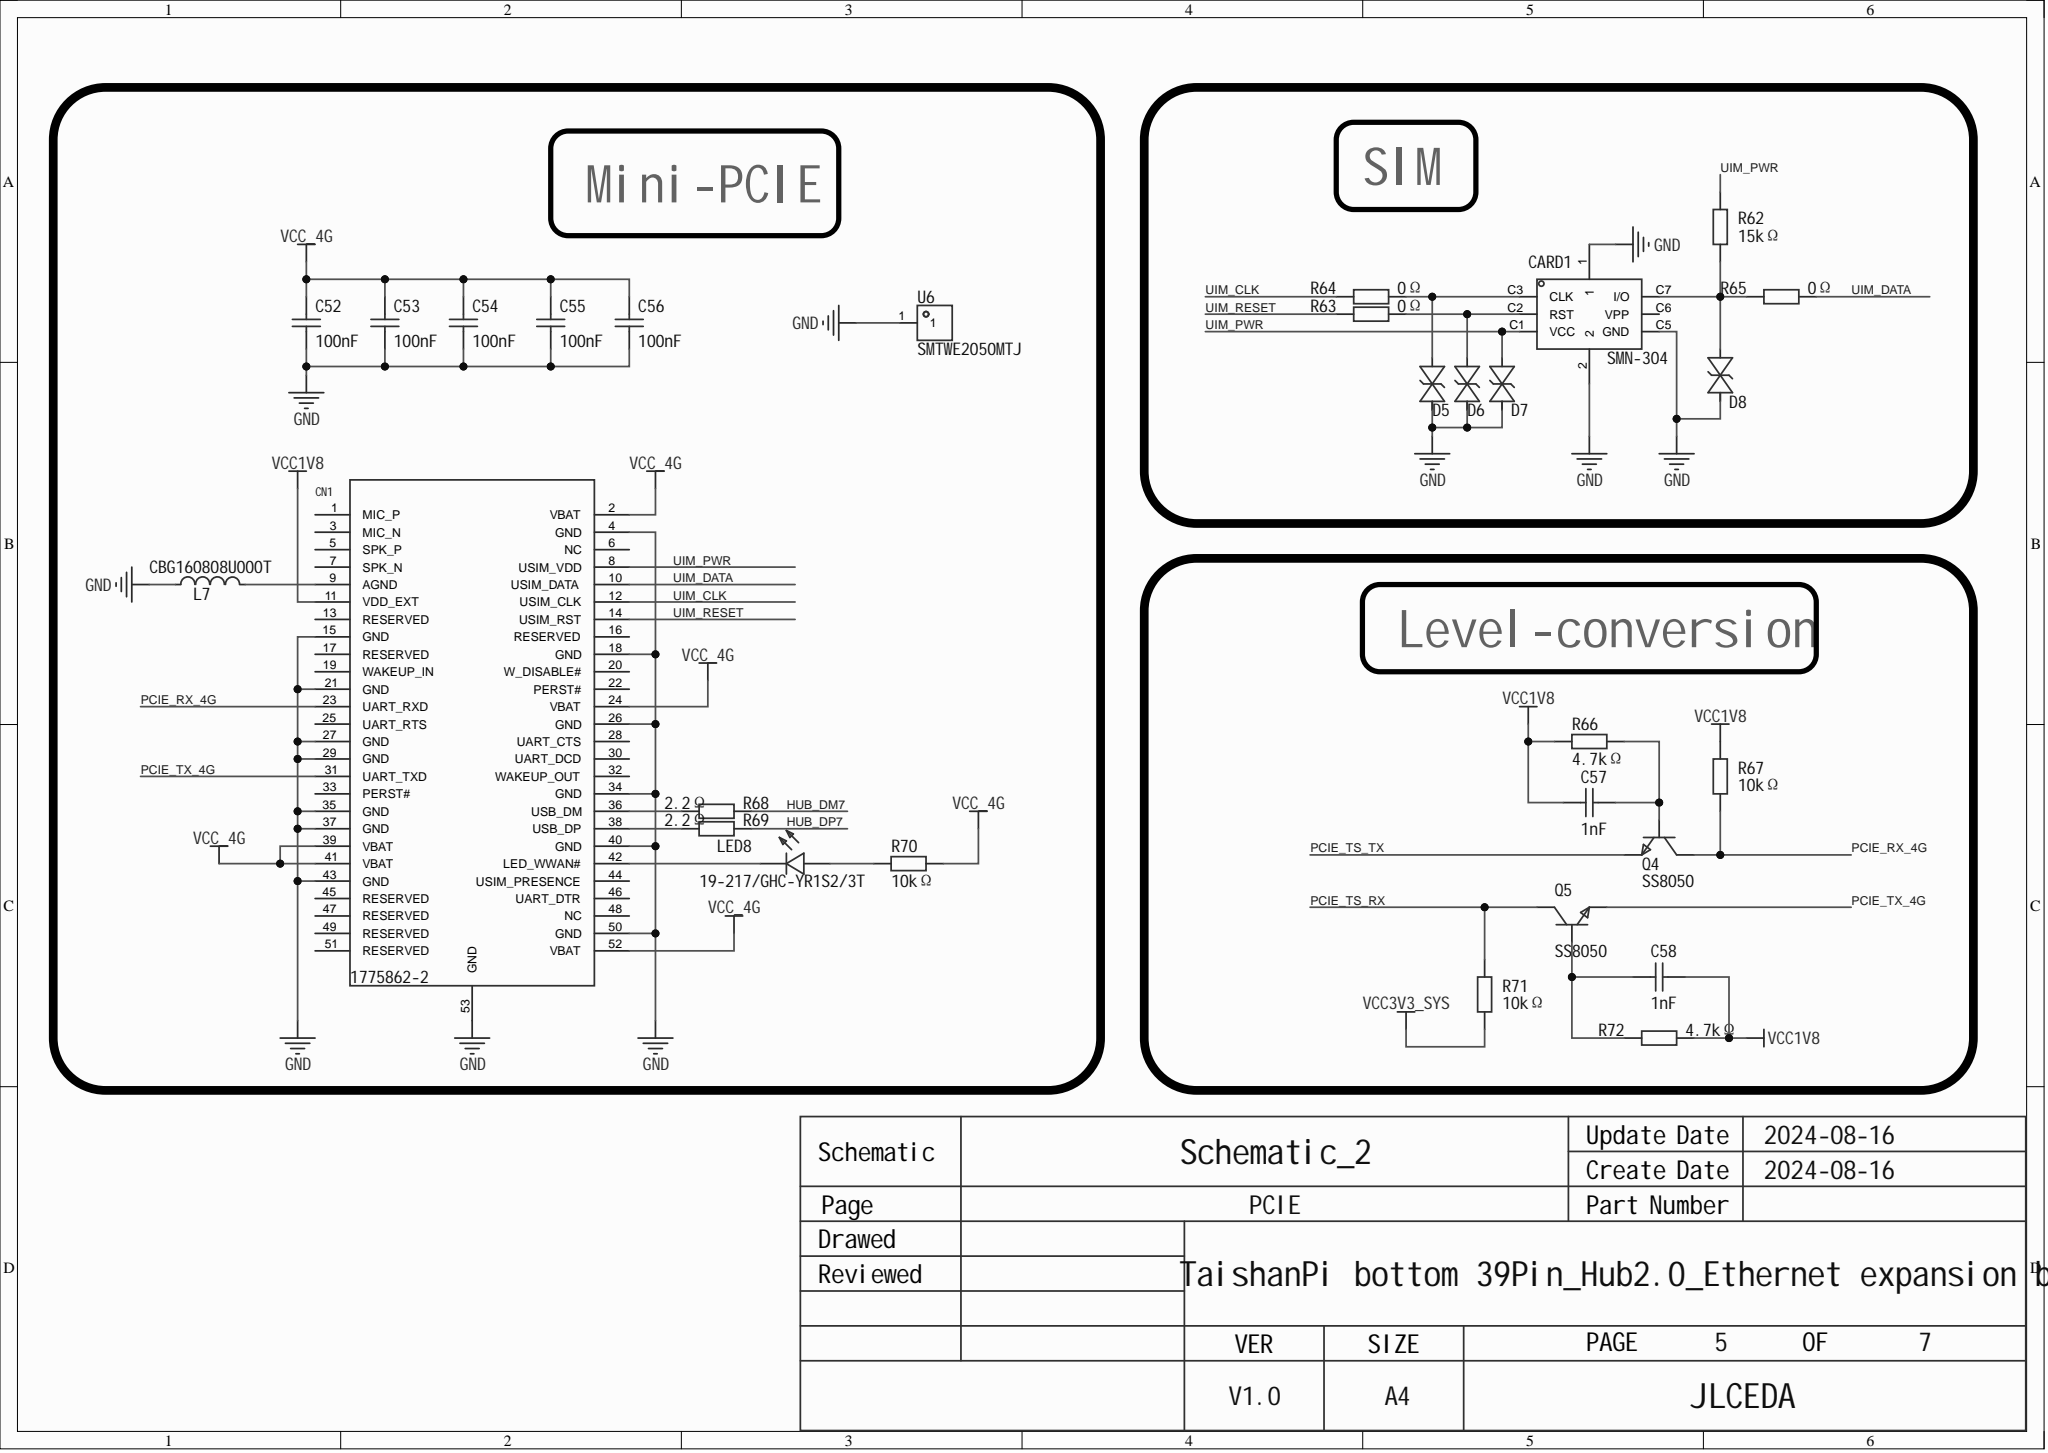Circuit board | Altium Designer | 209 parts | 149 nets | one sheet of the schematic
Parts on this sheet (reference | value | footprint):
C52 | 100nF | R0402
C53 | 100nF | R0402
C54 | 100nF | R0402
C55 | 100nF | R0402
C56 | 100nF | R0402
C57 | 1nF | R0402
C58 | 1nF | R0402
CARD1 | SMN-304 | SIM-SMD_SMN-304
CN1 | 1775862-2 | PCI-SMD_1775862-2
D5 | KLXES15AAA1 | R0402
D6 | KLXES15AAA1 | R0402
D7 | KLXES15AAA1 | R0402
D8 | KLXES15AAA1 | R0402
L7 | CBG160808U000T | L0603
LED8 | 19-217/GHC-YR1S2/3T | LED0603-RD
Q4 | SS8050 | SOT-23-3_L2.9-W1.3-P1.90-LS2.4-BR
Q5 | SS8050 | SOT-23-3_L2.9-W1.3-P1.90-LS2.4-BR
R62 | 15kΩ | R0402
R63 | 0Ω | R0402
R64 | 0Ω | R0402
R65 | 0Ω | R0402
R66 | 4.7kΩ | R0402
R67 | 10kΩ | R0402
R68 | 2.2Ω | R0402
R69 | 2.2Ω | R0402
R70 | 10kΩ | R0402
R71 | 10kΩ | R0402
R72 | 4.7kΩ | R0402
U6 | SMTWE2050MTJ | SMD_BD4.4-L4.4-D2.8
Nets of these parts (net: part-pin ...):
VCC_4G: C52-2 C53-2 C54-2 C55-2 C56-2 R70-2 CN1-2 CN1-24 CN1-39 CN1-41 CN1-52
VCC3V3_SYS: R71-1
VCC1V8: C57-1 C58-2 R66-1 R67-2 R72-2 CN1-11
UIM_RESET: R63-1 CN1-14
UIM_PWR: CARD1-C1 D7-1 R62-2 CN1-8
UIM_DATA: R65-2 CN1-10
UIM_CLK: R64-1 CN1-12
PCIE_TX_4G: Q5-2 CN1-31
PCIE_TS_TX: Q4-2
PCIE_TS_RX: Q5-3 R71-2
PCIE_RX_4G: Q4-3 R67-1 CN1-23
NetLED8_2: LED8-2 R70-1
NetCN1_42: LED8-1 CN1-42
NetCN1_38: R69-1 CN1-38
NetCN1_36: R68-1 CN1-36
NetCN1_9: L7-2 CN1-9
NetCARD1_C7: CARD1-C7 D8-1 R62-1 R65-1
NetCARD1_C3: CARD1-C3 D5-1 R64-2
NetCARD1_C2: CARD1-C2 D6-1 R63-2
NetC58_1: C58-1 Q5-1 R72-1
NetC57_2: C57-2 Q4-1 R66-2
HUB_DP7: R69-2
HUB_DM7: R68-2
GND: C52-1 C53-1 C54-1 C55-1 C56-1 CARD1-1 CARD1-2 CARD1-C5 D5-2 D6-2 D7-2 D8-2 L7-1 U6-1 CN1-4 CN1-15 CN1-18 CN1-21 CN1-26 CN1-27 CN1-29 CN1-34 CN1-35 CN1-37 CN1-40 CN1-43 CN1-50 CN1-53